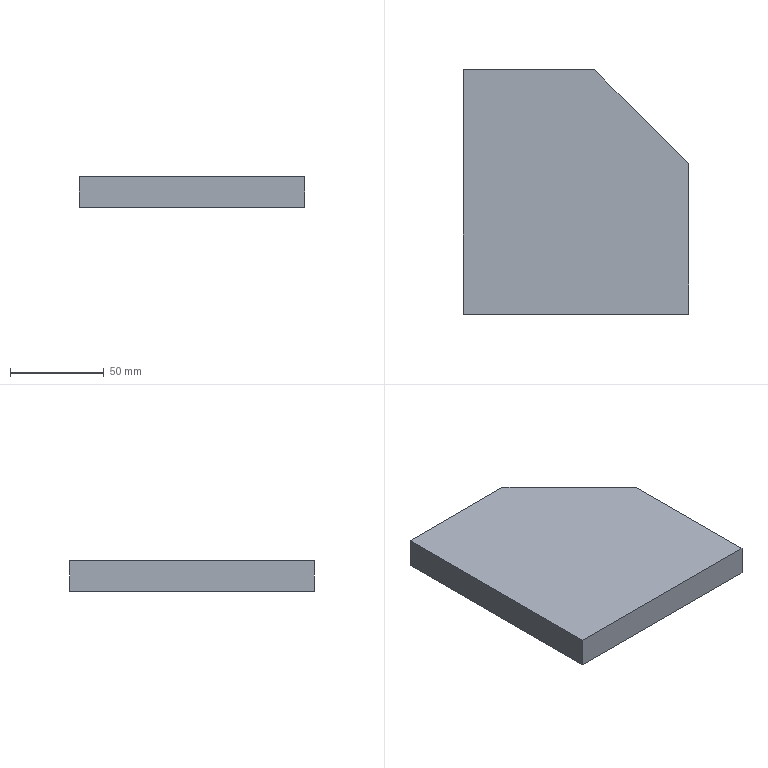Part | SolidWorks | features Chamfer 1, Extrusion 1 | 1 solid | 7 faces | box 120 x 130 x 16 mm | volume 229600 mm3 | plane 7
STEP:
#1=CARTESIAN_POINT('',(70.,130.,8.));
#2=VERTEX_POINT('',#1);
#3=CARTESIAN_POINT('',(0.,130.,8.));
#4=VERTEX_POINT('',#3);
#5=CARTESIAN_POINT('',(120.,130.,8.));
#6=DIRECTION('',(-1.,0.,0.));
#7=VECTOR('',#6,1000.);
#8=LINE('',#5,#7);
#9=EDGE_CURVE('',#2,#4,#8,.T.);
#10=ORIENTED_EDGE('',*,*,#9,.F.);
#11=CARTESIAN_POINT('',(70.,130.,-8.));
#12=VERTEX_POINT('',#11);
#13=CARTESIAN_POINT('',(70.,130.,8.));
#14=DIRECTION('',(0.,0.,-1.));
#15=VECTOR('',#14,1000.);
#16=LINE('',#13,#15);
#17=EDGE_CURVE('',#2,#12,#16,.T.);
#18=ORIENTED_EDGE('',*,*,#17,.T.);
#19=CARTESIAN_POINT('',(0.,130.,-8.));
#20=VERTEX_POINT('',#19);
#21=CARTESIAN_POINT('',(120.,130.,-8.));
#22=DIRECTION('',(-1.,0.,0.));
#23=VECTOR('',#22,1000.);
#24=LINE('',#21,#23);
#25=EDGE_CURVE('',#12,#20,#24,.T.);
#26=ORIENTED_EDGE('',*,*,#25,.T.);
#27=CARTESIAN_POINT('',(0.,130.,8.));
#28=DIRECTION('',(0.,0.,-1.));
#29=VECTOR('',#28,1000.);
#30=LINE('',#27,#29);
#31=EDGE_CURVE('',#4,#20,#30,.T.);
#32=ORIENTED_EDGE('',*,*,#31,.F.);
#33=EDGE_LOOP('',(#10,#18,#26,#32));
#34=FACE_OUTER_BOUND('',#33,.T.);
#35=CARTESIAN_POINT('',(120.,130.,8.));
#36=DIRECTION('',(0.,-1.,0.));
#37=DIRECTION('',(1.,0.,0.));
#38=AXIS2_PLACEMENT_3D('',#35,#36,#37);
#39=PLANE('',#38);
#40=ADVANCED_FACE('',(#34),#39,.F.);
#41=CARTESIAN_POINT('',(0.,0.,-8.));
#42=VERTEX_POINT('',#41);
#43=CARTESIAN_POINT('',(0.,130.,-8.));
#44=DIRECTION('',(0.,-1.,0.));
#45=VECTOR('',#44,1000.);
#46=LINE('',#43,#45);
#47=EDGE_CURVE('',#20,#42,#46,.T.);
#48=ORIENTED_EDGE('',*,*,#47,.T.);
#49=CARTESIAN_POINT('',(0.,0.,8.));
#50=VERTEX_POINT('',#49);
#51=CARTESIAN_POINT('',(0.,0.,8.));
#52=DIRECTION('',(0.,0.,-1.));
#53=VECTOR('',#52,1000.);
#54=LINE('',#51,#53);
#55=EDGE_CURVE('',#50,#42,#54,.T.);
#56=ORIENTED_EDGE('',*,*,#55,.F.);
#57=CARTESIAN_POINT('',(0.,130.,8.));
#58=DIRECTION('',(0.,-1.,0.));
#59=VECTOR('',#58,1000.);
#60=LINE('',#57,#59);
#61=EDGE_CURVE('',#4,#50,#60,.T.);
#62=ORIENTED_EDGE('',*,*,#61,.F.);
#63=ORIENTED_EDGE('',*,*,#31,.T.);
#64=EDGE_LOOP('',(#48,#56,#62,#63));
#65=FACE_OUTER_BOUND('',#64,.T.);
#66=CARTESIAN_POINT('',(0.,130.,8.));
#67=DIRECTION('',(1.,0.,0.));
#68=DIRECTION('',(0.,1.,0.));
#69=AXIS2_PLACEMENT_3D('',#66,#67,#68);
#70=PLANE('',#69);
#71=ADVANCED_FACE('',(#65),#70,.F.);
#72=CARTESIAN_POINT('',(120.,0.,-8.));
#73=VERTEX_POINT('',#72);
#74=CARTESIAN_POINT('',(0.,0.,-8.));
#75=DIRECTION('',(1.,0.,0.));
#76=VECTOR('',#75,1000.);
#77=LINE('',#74,#76);
#78=EDGE_CURVE('',#42,#73,#77,.T.);
#79=ORIENTED_EDGE('',*,*,#78,.T.);
#80=CARTESIAN_POINT('',(120.,0.,8.));
#81=VERTEX_POINT('',#80);
#82=CARTESIAN_POINT('',(120.,0.,8.));
#83=DIRECTION('',(0.,0.,-1.));
#84=VECTOR('',#83,1000.);
#85=LINE('',#82,#84);
#86=EDGE_CURVE('',#81,#73,#85,.T.);
#87=ORIENTED_EDGE('',*,*,#86,.F.);
#88=CARTESIAN_POINT('',(0.,0.,8.));
#89=DIRECTION('',(1.,0.,0.));
#90=VECTOR('',#89,1000.);
#91=LINE('',#88,#90);
#92=EDGE_CURVE('',#50,#81,#91,.T.);
#93=ORIENTED_EDGE('',*,*,#92,.F.);
#94=ORIENTED_EDGE('',*,*,#55,.T.);
#95=EDGE_LOOP('',(#79,#87,#93,#94));
#96=FACE_OUTER_BOUND('',#95,.T.);
#97=CARTESIAN_POINT('',(0.,0.,8.));
#98=DIRECTION('',(0.,1.,0.));
#99=DIRECTION('',(0.,0.,1.));
#100=AXIS2_PLACEMENT_3D('',#97,#98,#99);
#101=PLANE('',#100);
#102=ADVANCED_FACE('',(#96),#101,.F.);
#103=CARTESIAN_POINT('',(120.,80.,-8.));
#104=VERTEX_POINT('',#103);
#105=CARTESIAN_POINT('',(120.,0.,-8.));
#106=DIRECTION('',(0.,1.,0.));
#107=VECTOR('',#106,1000.);
#108=LINE('',#105,#107);
#109=EDGE_CURVE('',#73,#104,#108,.T.);
#110=ORIENTED_EDGE('',*,*,#109,.T.);
#111=CARTESIAN_POINT('',(120.,80.,8.));
#112=VERTEX_POINT('',#111);
#113=CARTESIAN_POINT('',(120.,80.,8.));
#114=DIRECTION('',(0.,0.,1.));
#115=VECTOR('',#114,1000.);
#116=LINE('',#113,#115);
#117=EDGE_CURVE('',#104,#112,#116,.T.);
#118=ORIENTED_EDGE('',*,*,#117,.T.);
#119=CARTESIAN_POINT('',(120.,0.,8.));
#120=DIRECTION('',(0.,1.,0.));
#121=VECTOR('',#120,1000.);
#122=LINE('',#119,#121);
#123=EDGE_CURVE('',#81,#112,#122,.T.);
#124=ORIENTED_EDGE('',*,*,#123,.F.);
#125=ORIENTED_EDGE('',*,*,#86,.T.);
#126=EDGE_LOOP('',(#110,#118,#124,#125));
#127=FACE_OUTER_BOUND('',#126,.T.);
#128=CARTESIAN_POINT('',(120.,0.,8.));
#129=DIRECTION('',(-1.,0.,0.));
#130=DIRECTION('',(0.,-1.,0.));
#131=AXIS2_PLACEMENT_3D('',#128,#129,#130);
#132=PLANE('',#131);
#133=ADVANCED_FACE('',(#127),#132,.F.);
#134=ORIENTED_EDGE('',*,*,#123,.T.);
#135=CARTESIAN_POINT('',(100.,100.,8.));
#136=DIRECTION('',(-0.7071,0.7071,0.));
#137=VECTOR('',#136,1000.);
#138=LINE('',#135,#137);
#139=EDGE_CURVE('',#112,#2,#138,.T.);
#140=ORIENTED_EDGE('',*,*,#139,.T.);
#141=ORIENTED_EDGE('',*,*,#9,.T.);
#142=ORIENTED_EDGE('',*,*,#61,.T.);
#143=ORIENTED_EDGE('',*,*,#92,.T.);
#144=EDGE_LOOP('',(#134,#140,#141,#142,#143));
#145=FACE_OUTER_BOUND('',#144,.T.);
#146=CARTESIAN_POINT('',(0.,0.,8.));
#147=DIRECTION('',(0.,0.,1.));
#148=DIRECTION('',(1.,0.,0.));
#149=AXIS2_PLACEMENT_3D('',#146,#147,#148);
#150=PLANE('',#149);
#151=ADVANCED_FACE('',(#145),#150,.T.);
#152=ORIENTED_EDGE('',*,*,#25,.F.);
#153=CARTESIAN_POINT('',(70.,130.,-8.));
#154=DIRECTION('',(0.7071,-0.7071,0.));
#155=VECTOR('',#154,1000.);
#156=LINE('',#153,#155);
#157=EDGE_CURVE('',#12,#104,#156,.T.);
#158=ORIENTED_EDGE('',*,*,#157,.T.);
#159=ORIENTED_EDGE('',*,*,#109,.F.);
#160=ORIENTED_EDGE('',*,*,#78,.F.);
#161=ORIENTED_EDGE('',*,*,#47,.F.);
#162=EDGE_LOOP('',(#152,#158,#159,#160,#161));
#163=FACE_OUTER_BOUND('',#162,.T.);
#164=CARTESIAN_POINT('',(0.,0.,-8.));
#165=DIRECTION('',(0.,0.,1.));
#166=DIRECTION('',(1.,0.,0.));
#167=AXIS2_PLACEMENT_3D('',#164,#165,#166);
#168=PLANE('',#167);
#169=ADVANCED_FACE('',(#163),#168,.F.);
#170=ORIENTED_EDGE('',*,*,#139,.F.);
#171=ORIENTED_EDGE('',*,*,#117,.F.);
#172=ORIENTED_EDGE('',*,*,#157,.F.);
#173=ORIENTED_EDGE('',*,*,#17,.F.);
#174=EDGE_LOOP('',(#170,#171,#172,#173));
#175=FACE_OUTER_BOUND('',#174,.T.);
#176=CARTESIAN_POINT('',(70.,130.,8.));
#177=DIRECTION('',(-0.7071,-0.7071,0.));
#178=DIRECTION('',(0.,0.,-1.));
#179=AXIS2_PLACEMENT_3D('',#176,#177,#178);
#180=PLANE('',#179);
#181=ADVANCED_FACE('',(#175),#180,.F.);
#182=CLOSED_SHELL('',(#40,#71,#102,#133,#151,#169,#181));
#183=MANIFOLD_SOLID_BREP('',#182);
#184=CARTESIAN_POINT('',(0.,0.,0.));
#185=DIRECTION('',(0.,0.,1.));
#186=DIRECTION('',(1.,0.,0.));
#187=AXIS2_PLACEMENT_3D('',#184,#185,#186);
#188=(LENGTH_UNIT()NAMED_UNIT(*)SI_UNIT(.MILLI.,.METRE.));
#189=UNCERTAINTY_MEASURE_WITH_UNIT(LENGTH_MEASURE(0.00001),#188,'','');
#190=(NAMED_UNIT(*)PLANE_ANGLE_UNIT()SI_UNIT($,.RADIAN.));
#191=(NAMED_UNIT(*)SI_UNIT($,.STERADIAN.)SOLID_ANGLE_UNIT());
#192=(GEOMETRIC_REPRESENTATION_CONTEXT(3)GLOBAL_UNCERTAINTY_ASSIGNED_CONTEXT((#189))GLOBAL_UNIT_ASSIGNED_CONTEXT((#188,#190,#191))REPRESENTATION_CONTEXT('',''));
#193=ADVANCED_BREP_SHAPE_REPRESENTATION('',(#183,#187),#192);